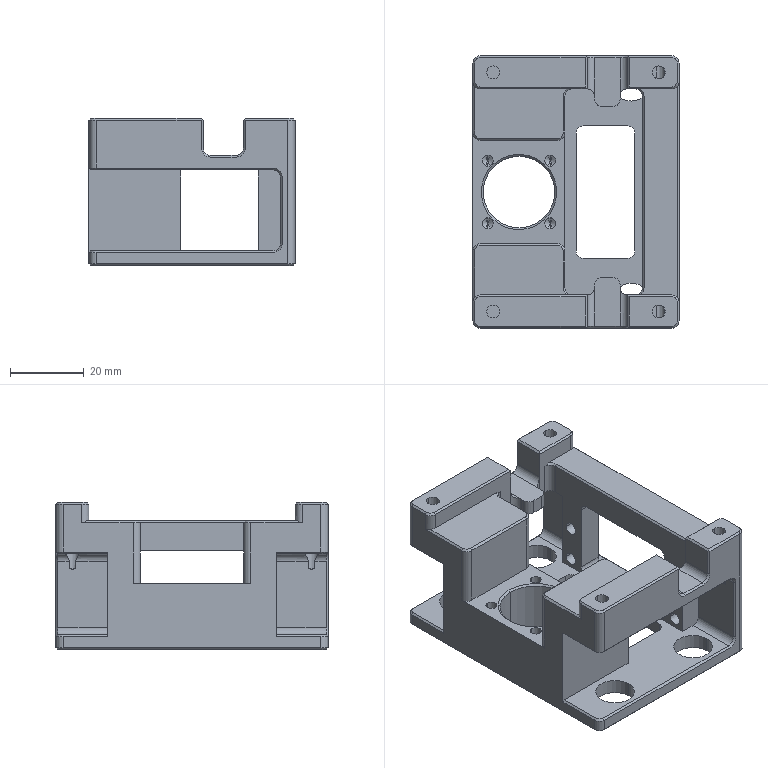Part | 1 solid | 247 faces | box 56 x 74 x 40 mm | volume 53067 mm3 | plane 107 | cylinder 82 | cone 58 | commonest cylinder face diameters 4 x48 3.5 x16 3 x8 10.5 x8 19.5 x2